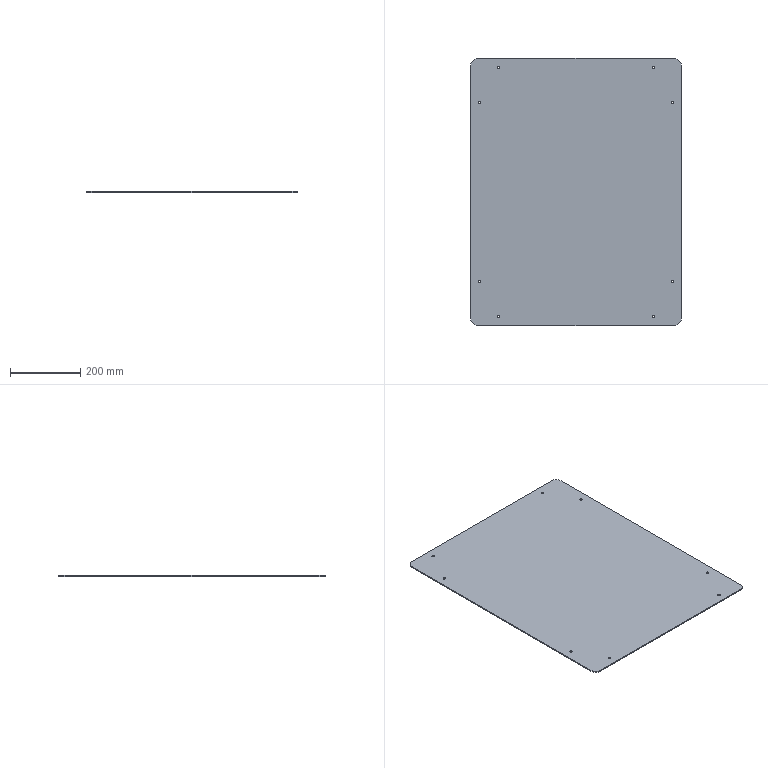Part | STEP file | 11-yakeli11 | 1 solid | 26 faces | box 600 x 760 x 3 mm | volume 1366046 mm3 | cylinder 20 | plane 6 | commonest cylinder face diameters 7 x16 40 x4
STEP:
#1=CARTESIAN_POINT('',(-216.5,-355.,0.));
#2=VERTEX_POINT('',#1);
#3=CARTESIAN_POINT('',(-223.5,-355.,0.));
#4=VERTEX_POINT('',#3);
#5=CARTESIAN_POINT('',(-220.,-355.,0.));
#6=DIRECTION('',(0.,0.,-1.));
#7=DIRECTION('',(1.,0.,0.));
#8=AXIS2_PLACEMENT_3D('',#5,#6,#7);
#9=CIRCLE('',#8,3.5);
#10=EDGE_CURVE('',#2,#4,#9,.T.);
#11=ORIENTED_EDGE('',*,*,#10,.F.);
#12=CARTESIAN_POINT('',(-216.5,-355.,-3.));
#13=VERTEX_POINT('',#12);
#14=CARTESIAN_POINT('',(-216.5,-355.,0.));
#15=DIRECTION('',(0.,0.,-1.));
#16=VECTOR('',#15,1000.);
#17=LINE('',#14,#16);
#18=EDGE_CURVE('',#2,#13,#17,.T.);
#19=ORIENTED_EDGE('',*,*,#18,.T.);
#20=CARTESIAN_POINT('',(-223.5,-355.,-3.));
#21=VERTEX_POINT('',#20);
#22=CARTESIAN_POINT('',(-220.,-355.,-3.));
#23=DIRECTION('',(0.,0.,-1.));
#24=DIRECTION('',(1.,0.,0.));
#25=AXIS2_PLACEMENT_3D('',#22,#23,#24);
#26=CIRCLE('',#25,3.5);
#27=EDGE_CURVE('',#13,#21,#26,.T.);
#28=ORIENTED_EDGE('',*,*,#27,.T.);
#29=CARTESIAN_POINT('',(-223.5,-355.,0.));
#30=DIRECTION('',(0.,0.,-1.));
#31=VECTOR('',#30,1000.);
#32=LINE('',#29,#31);
#33=EDGE_CURVE('',#4,#21,#32,.T.);
#34=ORIENTED_EDGE('',*,*,#33,.F.);
#35=EDGE_LOOP('',(#11,#19,#28,#34));
#36=FACE_OUTER_BOUND('',#35,.T.);
#37=CARTESIAN_POINT('',(-220.,-355.,0.));
#38=DIRECTION('',(0.,0.,-1.));
#39=DIRECTION('',(-1.,0.,0.));
#40=AXIS2_PLACEMENT_3D('',#37,#38,#39);
#41=CYLINDRICAL_SURFACE('',#40,3.5);
#42=ADVANCED_FACE('',(#36),#41,.F.);
#43=CARTESIAN_POINT('',(223.5,-355.,0.));
#44=VERTEX_POINT('',#43);
#45=CARTESIAN_POINT('',(216.5,-355.,0.));
#46=VERTEX_POINT('',#45);
#47=CARTESIAN_POINT('',(220.,-355.,0.));
#48=DIRECTION('',(0.,0.,-1.));
#49=DIRECTION('',(1.,0.,0.));
#50=AXIS2_PLACEMENT_3D('',#47,#48,#49);
#51=CIRCLE('',#50,3.5);
#52=EDGE_CURVE('',#44,#46,#51,.T.);
#53=ORIENTED_EDGE('',*,*,#52,.F.);
#54=CARTESIAN_POINT('',(223.5,-355.,-3.));
#55=VERTEX_POINT('',#54);
#56=CARTESIAN_POINT('',(223.5,-355.,0.));
#57=DIRECTION('',(0.,0.,-1.));
#58=VECTOR('',#57,1000.);
#59=LINE('',#56,#58);
#60=EDGE_CURVE('',#44,#55,#59,.T.);
#61=ORIENTED_EDGE('',*,*,#60,.T.);
#62=CARTESIAN_POINT('',(216.5,-355.,-3.));
#63=VERTEX_POINT('',#62);
#64=CARTESIAN_POINT('',(220.,-355.,-3.));
#65=DIRECTION('',(0.,0.,-1.));
#66=DIRECTION('',(1.,0.,0.));
#67=AXIS2_PLACEMENT_3D('',#64,#65,#66);
#68=CIRCLE('',#67,3.5);
#69=EDGE_CURVE('',#55,#63,#68,.T.);
#70=ORIENTED_EDGE('',*,*,#69,.T.);
#71=CARTESIAN_POINT('',(216.5,-355.,0.));
#72=DIRECTION('',(0.,0.,-1.));
#73=VECTOR('',#72,1000.);
#74=LINE('',#71,#73);
#75=EDGE_CURVE('',#46,#63,#74,.T.);
#76=ORIENTED_EDGE('',*,*,#75,.F.);
#77=EDGE_LOOP('',(#53,#61,#70,#76));
#78=FACE_OUTER_BOUND('',#77,.T.);
#79=CARTESIAN_POINT('',(220.,-355.,0.));
#80=DIRECTION('',(0.,0.,-1.));
#81=DIRECTION('',(-1.,0.,0.));
#82=AXIS2_PLACEMENT_3D('',#79,#80,#81);
#83=CYLINDRICAL_SURFACE('',#82,3.5);
#84=ADVANCED_FACE('',(#78),#83,.F.);
#85=CARTESIAN_POINT('',(223.5,355.,0.));
#86=VERTEX_POINT('',#85);
#87=CARTESIAN_POINT('',(216.5,355.,0.));
#88=VERTEX_POINT('',#87);
#89=CARTESIAN_POINT('',(220.,355.,0.));
#90=DIRECTION('',(0.,0.,-1.));
#91=DIRECTION('',(-1.,0.,0.));
#92=AXIS2_PLACEMENT_3D('',#89,#90,#91);
#93=CIRCLE('',#92,3.5);
#94=EDGE_CURVE('',#86,#88,#93,.T.);
#95=ORIENTED_EDGE('',*,*,#94,.F.);
#96=CARTESIAN_POINT('',(223.5,355.,-3.));
#97=VERTEX_POINT('',#96);
#98=CARTESIAN_POINT('',(223.5,355.,0.));
#99=DIRECTION('',(0.,0.,-1.));
#100=VECTOR('',#99,1000.);
#101=LINE('',#98,#100);
#102=EDGE_CURVE('',#86,#97,#101,.T.);
#103=ORIENTED_EDGE('',*,*,#102,.T.);
#104=CARTESIAN_POINT('',(216.5,355.,-3.));
#105=VERTEX_POINT('',#104);
#106=CARTESIAN_POINT('',(220.,355.,-3.));
#107=DIRECTION('',(0.,0.,-1.));
#108=DIRECTION('',(-1.,0.,0.));
#109=AXIS2_PLACEMENT_3D('',#106,#107,#108);
#110=CIRCLE('',#109,3.5);
#111=EDGE_CURVE('',#97,#105,#110,.T.);
#112=ORIENTED_EDGE('',*,*,#111,.T.);
#113=CARTESIAN_POINT('',(216.5,355.,0.));
#114=DIRECTION('',(0.,0.,-1.));
#115=VECTOR('',#114,1000.);
#116=LINE('',#113,#115);
#117=EDGE_CURVE('',#88,#105,#116,.T.);
#118=ORIENTED_EDGE('',*,*,#117,.F.);
#119=EDGE_LOOP('',(#95,#103,#112,#118));
#120=FACE_OUTER_BOUND('',#119,.T.);
#121=CARTESIAN_POINT('',(220.,355.,0.));
#122=DIRECTION('',(0.,0.,-1.));
#123=DIRECTION('',(-1.,0.,0.));
#124=AXIS2_PLACEMENT_3D('',#121,#122,#123);
#125=CYLINDRICAL_SURFACE('',#124,3.5);
#126=ADVANCED_FACE('',(#120),#125,.F.);
#127=CARTESIAN_POINT('',(-216.5,355.,0.));
#128=VERTEX_POINT('',#127);
#129=CARTESIAN_POINT('',(-223.5,355.,0.));
#130=VERTEX_POINT('',#129);
#131=CARTESIAN_POINT('',(-220.,355.,0.));
#132=DIRECTION('',(0.,0.,-1.));
#133=DIRECTION('',(-1.,0.,0.));
#134=AXIS2_PLACEMENT_3D('',#131,#132,#133);
#135=CIRCLE('',#134,3.5);
#136=EDGE_CURVE('',#128,#130,#135,.T.);
#137=ORIENTED_EDGE('',*,*,#136,.F.);
#138=CARTESIAN_POINT('',(-216.5,355.,-3.));
#139=VERTEX_POINT('',#138);
#140=CARTESIAN_POINT('',(-216.5,355.,0.));
#141=DIRECTION('',(0.,0.,-1.));
#142=VECTOR('',#141,1000.);
#143=LINE('',#140,#142);
#144=EDGE_CURVE('',#128,#139,#143,.T.);
#145=ORIENTED_EDGE('',*,*,#144,.T.);
#146=CARTESIAN_POINT('',(-223.5,355.,-3.));
#147=VERTEX_POINT('',#146);
#148=CARTESIAN_POINT('',(-220.,355.,-3.));
#149=DIRECTION('',(0.,0.,-1.));
#150=DIRECTION('',(-1.,0.,0.));
#151=AXIS2_PLACEMENT_3D('',#148,#149,#150);
#152=CIRCLE('',#151,3.5);
#153=EDGE_CURVE('',#139,#147,#152,.T.);
#154=ORIENTED_EDGE('',*,*,#153,.T.);
#155=CARTESIAN_POINT('',(-223.5,355.,0.));
#156=DIRECTION('',(0.,0.,-1.));
#157=VECTOR('',#156,1000.);
#158=LINE('',#155,#157);
#159=EDGE_CURVE('',#130,#147,#158,.T.);
#160=ORIENTED_EDGE('',*,*,#159,.F.);
#161=EDGE_LOOP('',(#137,#145,#154,#160));
#162=FACE_OUTER_BOUND('',#161,.T.);
#163=CARTESIAN_POINT('',(-220.,355.,0.));
#164=DIRECTION('',(0.,0.,-1.));
#165=DIRECTION('',(-1.,0.,0.));
#166=AXIS2_PLACEMENT_3D('',#163,#164,#165);
#167=CYLINDRICAL_SURFACE('',#166,3.5);
#168=ADVANCED_FACE('',(#162),#167,.F.);
#169=CARTESIAN_POINT('',(278.5,255.,0.));
#170=VERTEX_POINT('',#169);
#171=CARTESIAN_POINT('',(271.5,255.,0.));
#172=VERTEX_POINT('',#171);
#173=CARTESIAN_POINT('',(275.,255.,0.));
#174=DIRECTION('',(0.,0.,-1.));
#175=DIRECTION('',(-1.,0.,0.));
#176=AXIS2_PLACEMENT_3D('',#173,#174,#175);
#177=CIRCLE('',#176,3.5);
#178=EDGE_CURVE('',#170,#172,#177,.T.);
#179=ORIENTED_EDGE('',*,*,#178,.F.);
#180=CARTESIAN_POINT('',(278.5,255.,-3.));
#181=VERTEX_POINT('',#180);
#182=CARTESIAN_POINT('',(278.5,255.,0.));
#183=DIRECTION('',(0.,0.,-1.));
#184=VECTOR('',#183,1000.);
#185=LINE('',#182,#184);
#186=EDGE_CURVE('',#170,#181,#185,.T.);
#187=ORIENTED_EDGE('',*,*,#186,.T.);
#188=CARTESIAN_POINT('',(271.5,255.,-3.));
#189=VERTEX_POINT('',#188);
#190=CARTESIAN_POINT('',(275.,255.,-3.));
#191=DIRECTION('',(0.,0.,-1.));
#192=DIRECTION('',(-1.,0.,0.));
#193=AXIS2_PLACEMENT_3D('',#190,#191,#192);
#194=CIRCLE('',#193,3.5);
#195=EDGE_CURVE('',#181,#189,#194,.T.);
#196=ORIENTED_EDGE('',*,*,#195,.T.);
#197=CARTESIAN_POINT('',(271.5,255.,0.));
#198=DIRECTION('',(0.,0.,-1.));
#199=VECTOR('',#198,1000.);
#200=LINE('',#197,#199);
#201=EDGE_CURVE('',#172,#189,#200,.T.);
#202=ORIENTED_EDGE('',*,*,#201,.F.);
#203=EDGE_LOOP('',(#179,#187,#196,#202));
#204=FACE_OUTER_BOUND('',#203,.T.);
#205=CARTESIAN_POINT('',(275.,255.,0.));
#206=DIRECTION('',(0.,0.,-1.));
#207=DIRECTION('',(-1.,0.,0.));
#208=AXIS2_PLACEMENT_3D('',#205,#206,#207);
#209=CYLINDRICAL_SURFACE('',#208,3.5);
#210=ADVANCED_FACE('',(#204),#209,.F.);
#211=CARTESIAN_POINT('',(278.5,-255.,0.));
#212=VERTEX_POINT('',#211);
#213=CARTESIAN_POINT('',(271.5,-255.,0.));
#214=VERTEX_POINT('',#213);
#215=CARTESIAN_POINT('',(275.,-255.,0.));
#216=DIRECTION('',(0.,0.,-1.));
#217=DIRECTION('',(-1.,0.,0.));
#218=AXIS2_PLACEMENT_3D('',#215,#216,#217);
#219=CIRCLE('',#218,3.5);
#220=EDGE_CURVE('',#212,#214,#219,.T.);
#221=ORIENTED_EDGE('',*,*,#220,.F.);
#222=CARTESIAN_POINT('',(278.5,-255.,-3.));
#223=VERTEX_POINT('',#222);
#224=CARTESIAN_POINT('',(278.5,-255.,0.));
#225=DIRECTION('',(0.,0.,-1.));
#226=VECTOR('',#225,1000.);
#227=LINE('',#224,#226);
#228=EDGE_CURVE('',#212,#223,#227,.T.);
#229=ORIENTED_EDGE('',*,*,#228,.T.);
#230=CARTESIAN_POINT('',(271.5,-255.,-3.));
#231=VERTEX_POINT('',#230);
#232=CARTESIAN_POINT('',(275.,-255.,-3.));
#233=DIRECTION('',(0.,0.,-1.));
#234=DIRECTION('',(-1.,0.,0.));
#235=AXIS2_PLACEMENT_3D('',#232,#233,#234);
#236=CIRCLE('',#235,3.5);
#237=EDGE_CURVE('',#223,#231,#236,.T.);
#238=ORIENTED_EDGE('',*,*,#237,.T.);
#239=CARTESIAN_POINT('',(271.5,-255.,0.));
#240=DIRECTION('',(0.,0.,-1.));
#241=VECTOR('',#240,1000.);
#242=LINE('',#239,#241);
#243=EDGE_CURVE('',#214,#231,#242,.T.);
#244=ORIENTED_EDGE('',*,*,#243,.F.);
#245=EDGE_LOOP('',(#221,#229,#238,#244));
#246=FACE_OUTER_BOUND('',#245,.T.);
#247=CARTESIAN_POINT('',(275.,-255.,0.));
#248=DIRECTION('',(0.,0.,-1.));
#249=DIRECTION('',(-1.,0.,0.));
#250=AXIS2_PLACEMENT_3D('',#247,#248,#249);
#251=CYLINDRICAL_SURFACE('',#250,3.5);
#252=ADVANCED_FACE('',(#246),#251,.F.);
#253=CARTESIAN_POINT('',(-271.5,-255.,0.));
#254=VERTEX_POINT('',#253);
#255=CARTESIAN_POINT('',(-278.5,-255.,0.));
#256=VERTEX_POINT('',#255);
#257=CARTESIAN_POINT('',(-275.,-255.,0.));
#258=DIRECTION('',(0.,0.,-1.));
#259=DIRECTION('',(-1.,0.,0.));
#260=AXIS2_PLACEMENT_3D('',#257,#258,#259);
#261=CIRCLE('',#260,3.5);
#262=EDGE_CURVE('',#254,#256,#261,.T.);
#263=ORIENTED_EDGE('',*,*,#262,.F.);
#264=CARTESIAN_POINT('',(-271.5,-255.,-3.));
#265=VERTEX_POINT('',#264);
#266=CARTESIAN_POINT('',(-271.5,-255.,0.));
#267=DIRECTION('',(0.,0.,-1.));
#268=VECTOR('',#267,1000.);
#269=LINE('',#266,#268);
#270=EDGE_CURVE('',#254,#265,#269,.T.);
#271=ORIENTED_EDGE('',*,*,#270,.T.);
#272=CARTESIAN_POINT('',(-278.5,-255.,-3.));
#273=VERTEX_POINT('',#272);
#274=CARTESIAN_POINT('',(-275.,-255.,-3.));
#275=DIRECTION('',(0.,0.,-1.));
#276=DIRECTION('',(-1.,0.,0.));
#277=AXIS2_PLACEMENT_3D('',#274,#275,#276);
#278=CIRCLE('',#277,3.5);
#279=EDGE_CURVE('',#265,#273,#278,.T.);
#280=ORIENTED_EDGE('',*,*,#279,.T.);
#281=CARTESIAN_POINT('',(-278.5,-255.,0.));
#282=DIRECTION('',(0.,0.,-1.));
#283=VECTOR('',#282,1000.);
#284=LINE('',#281,#283);
#285=EDGE_CURVE('',#256,#273,#284,.T.);
#286=ORIENTED_EDGE('',*,*,#285,.F.);
#287=EDGE_LOOP('',(#263,#271,#280,#286));
#288=FACE_OUTER_BOUND('',#287,.T.);
#289=CARTESIAN_POINT('',(-275.,-255.,0.));
#290=DIRECTION('',(0.,0.,-1.));
#291=DIRECTION('',(-1.,0.,0.));
#292=AXIS2_PLACEMENT_3D('',#289,#290,#291);
#293=CYLINDRICAL_SURFACE('',#292,3.5);
#294=ADVANCED_FACE('',(#288),#293,.F.);
#295=CARTESIAN_POINT('',(-271.5,255.,0.));
#296=VERTEX_POINT('',#295);
#297=CARTESIAN_POINT('',(-278.5,255.,0.));
#298=VERTEX_POINT('',#297);
#299=CARTESIAN_POINT('',(-275.,255.,0.));
#300=DIRECTION('',(0.,0.,-1.));
#301=DIRECTION('',(-1.,0.,0.));
#302=AXIS2_PLACEMENT_3D('',#299,#300,#301);
#303=CIRCLE('',#302,3.5);
#304=EDGE_CURVE('',#296,#298,#303,.T.);
#305=ORIENTED_EDGE('',*,*,#304,.F.);
#306=CARTESIAN_POINT('',(-271.5,255.,-3.));
#307=VERTEX_POINT('',#306);
#308=CARTESIAN_POINT('',(-271.5,255.,0.));
#309=DIRECTION('',(0.,0.,-1.));
#310=VECTOR('',#309,1000.);
#311=LINE('',#308,#310);
#312=EDGE_CURVE('',#296,#307,#311,.T.);
#313=ORIENTED_EDGE('',*,*,#312,.T.);
#314=CARTESIAN_POINT('',(-278.5,255.,-3.));
#315=VERTEX_POINT('',#314);
#316=CARTESIAN_POINT('',(-275.,255.,-3.));
#317=DIRECTION('',(0.,0.,-1.));
#318=DIRECTION('',(-1.,0.,0.));
#319=AXIS2_PLACEMENT_3D('',#316,#317,#318);
#320=CIRCLE('',#319,3.5);
#321=EDGE_CURVE('',#307,#315,#320,.T.);
#322=ORIENTED_EDGE('',*,*,#321,.T.);
#323=CARTESIAN_POINT('',(-278.5,255.,0.));
#324=DIRECTION('',(0.,0.,-1.));
#325=VECTOR('',#324,1000.);
#326=LINE('',#323,#325);
#327=EDGE_CURVE('',#298,#315,#326,.T.);
#328=ORIENTED_EDGE('',*,*,#327,.F.);
#329=EDGE_LOOP('',(#305,#313,#322,#328));
#330=FACE_OUTER_BOUND('',#329,.T.);
#331=CARTESIAN_POINT('',(-275.,255.,0.));
#332=DIRECTION('',(0.,0.,-1.));
#333=DIRECTION('',(-1.,0.,0.));
#334=AXIS2_PLACEMENT_3D('',#331,#332,#333);
#335=CYLINDRICAL_SURFACE('',#334,3.5);
#336=ADVANCED_FACE('',(#330),#335,.F.);
#337=CARTESIAN_POINT('',(300.,-360.,0.));
#338=VERTEX_POINT('',#337);
#339=CARTESIAN_POINT('',(300.,360.,0.));
#340=VERTEX_POINT('',#339);
#341=CARTESIAN_POINT('',(300.,380.,0.));
#342=DIRECTION('',(0.,1.,0.));
#343=VECTOR('',#342,1000.);
#344=LINE('',#341,#343);
#345=EDGE_CURVE('',#338,#340,#344,.T.);
#346=ORIENTED_EDGE('',*,*,#345,.F.);
#347=CARTESIAN_POINT('',(300.,-360.,-3.));
#348=VERTEX_POINT('',#347);
#349=CARTESIAN_POINT('',(300.,-360.,-3.));
#350=DIRECTION('',(0.,0.,-1.));
#351=VECTOR('',#350,1000.);
#352=LINE('',#349,#351);
#353=EDGE_CURVE('',#338,#348,#352,.T.);
#354=ORIENTED_EDGE('',*,*,#353,.T.);
#355=CARTESIAN_POINT('',(300.,360.,-3.));
#356=VERTEX_POINT('',#355);
#357=CARTESIAN_POINT('',(300.,380.,-3.));
#358=DIRECTION('',(0.,1.,0.));
#359=VECTOR('',#358,1000.);
#360=LINE('',#357,#359);
#361=EDGE_CURVE('',#348,#356,#360,.T.);
#362=ORIENTED_EDGE('',*,*,#361,.T.);
#363=CARTESIAN_POINT('',(300.,360.,-3.));
#364=DIRECTION('',(0.,0.,1.));
#365=VECTOR('',#364,1000.);
#366=LINE('',#363,#365);
#367=EDGE_CURVE('',#356,#340,#366,.T.);
#368=ORIENTED_EDGE('',*,*,#367,.T.);
#369=EDGE_LOOP('',(#346,#354,#362,#368));
#370=FACE_OUTER_BOUND('',#369,.T.);
#371=CARTESIAN_POINT('',(300.,380.,-3.));
#372=DIRECTION('',(1.,0.,0.));
#373=DIRECTION('',(0.,1.,0.));
#374=AXIS2_PLACEMENT_3D('',#371,#372,#373);
#375=PLANE('',#374);
#376=ADVANCED_FACE('',(#370),#375,.T.);
#377=CARTESIAN_POINT('',(-280.,-380.,0.));
#378=VERTEX_POINT('',#377);
#379=CARTESIAN_POINT('',(280.,-380.,0.));
#380=VERTEX_POINT('',#379);
#381=CARTESIAN_POINT('',(-300.,-380.,0.));
#382=DIRECTION('',(1.,0.,0.));
#383=VECTOR('',#382,1000.);
#384=LINE('',#381,#383);
#385=EDGE_CURVE('',#378,#380,#384,.T.);
#386=ORIENTED_EDGE('',*,*,#385,.F.);
#387=CARTESIAN_POINT('',(-280.,-380.,-3.));
#388=VERTEX_POINT('',#387);
#389=CARTESIAN_POINT('',(-280.,-380.,-3.));
#390=DIRECTION('',(0.,0.,-1.));
#391=VECTOR('',#390,1000.);
#392=LINE('',#389,#391);
#393=EDGE_CURVE('',#378,#388,#392,.T.);
#394=ORIENTED_EDGE('',*,*,#393,.T.);
#395=CARTESIAN_POINT('',(280.,-380.,-3.));
#396=VERTEX_POINT('',#395);
#397=CARTESIAN_POINT('',(-300.,-380.,-3.));
#398=DIRECTION('',(1.,0.,0.));
#399=VECTOR('',#398,1000.);
#400=LINE('',#397,#399);
#401=EDGE_CURVE('',#388,#396,#400,.T.);
#402=ORIENTED_EDGE('',*,*,#401,.T.);
#403=CARTESIAN_POINT('',(280.,-380.,-3.));
#404=DIRECTION('',(0.,0.,1.));
#405=VECTOR('',#404,1000.);
#406=LINE('',#403,#405);
#407=EDGE_CURVE('',#396,#380,#406,.T.);
#408=ORIENTED_EDGE('',*,*,#407,.T.);
#409=EDGE_LOOP('',(#386,#394,#402,#408));
#410=FACE_OUTER_BOUND('',#409,.T.);
#411=CARTESIAN_POINT('',(-300.,-380.,-3.));
#412=DIRECTION('',(0.,-1.,0.));
#413=DIRECTION('',(0.,0.,-1.));
#414=AXIS2_PLACEMENT_3D('',#411,#412,#413);
#415=PLANE('',#414);
#416=ADVANCED_FACE('',(#410),#415,.T.);
#417=CARTESIAN_POINT('',(-300.,360.,-3.));
#418=VERTEX_POINT('',#417);
#419=CARTESIAN_POINT('',(-300.,-360.,-3.));
#420=VERTEX_POINT('',#419);
#421=CARTESIAN_POINT('',(-300.,380.,-3.));
#422=DIRECTION('',(0.,-1.,0.));
#423=VECTOR('',#422,1000.);
#424=LINE('',#421,#423);
#425=EDGE_CURVE('',#418,#420,#424,.T.);
#426=ORIENTED_EDGE('',*,*,#425,.T.);
#427=CARTESIAN_POINT('',(-300.,-360.,0.));
#428=VERTEX_POINT('',#427);
#429=CARTESIAN_POINT('',(-300.,-360.,-3.));
#430=DIRECTION('',(0.,0.,1.));
#431=VECTOR('',#430,1000.);
#432=LINE('',#429,#431);
#433=EDGE_CURVE('',#420,#428,#432,.T.);
#434=ORIENTED_EDGE('',*,*,#433,.T.);
#435=CARTESIAN_POINT('',(-300.,360.,0.));
#436=VERTEX_POINT('',#435);
#437=CARTESIAN_POINT('',(-300.,380.,0.));
#438=DIRECTION('',(0.,-1.,0.));
#439=VECTOR('',#438,1000.);
#440=LINE('',#437,#439);
#441=EDGE_CURVE('',#436,#428,#440,.T.);
#442=ORIENTED_EDGE('',*,*,#441,.F.);
#443=CARTESIAN_POINT('',(-300.,360.,-3.));
#444=DIRECTION('',(0.,0.,-1.));
#445=VECTOR('',#444,1000.);
#446=LINE('',#443,#445);
#447=EDGE_CURVE('',#436,#418,#446,.T.);
#448=ORIENTED_EDGE('',*,*,#447,.T.);
#449=EDGE_LOOP('',(#426,#434,#442,#448));
#450=FACE_OUTER_BOUND('',#449,.T.);
#451=CARTESIAN_POINT('',(-300.,380.,-3.));
#452=DIRECTION('',(-1.,0.,0.));
#453=DIRECTION('',(0.,-1.,0.));
#454=AXIS2_PLACEMENT_3D('',#451,#452,#453);
#455=PLANE('',#454);
#456=ADVANCED_FACE('',(#450),#455,.T.);
#457=CARTESIAN_POINT('',(280.,380.,0.));
#458=VERTEX_POINT('',#457);
#459=CARTESIAN_POINT('',(-280.,380.,0.));
#460=VERTEX_POINT('',#459);
#461=CARTESIAN_POINT('',(-300.,380.,0.));
#462=DIRECTION('',(-1.,0.,0.));
#463=VECTOR('',#462,1000.);
#464=LINE('',#461,#463);
#465=EDGE_CURVE('',#458,#460,#464,.T.);
#466=ORIENTED_EDGE('',*,*,#465,.F.);
#467=CARTESIAN_POINT('',(280.,380.,-3.));
#468=VERTEX_POINT('',#467);
#469=CARTESIAN_POINT('',(280.,380.,-3.));
#470=DIRECTION('',(0.,0.,-1.));
#471=VECTOR('',#470,1000.);
#472=LINE('',#469,#471);
#473=EDGE_CURVE('',#458,#468,#472,.T.);
#474=ORIENTED_EDGE('',*,*,#473,.T.);
#475=CARTESIAN_POINT('',(-280.,380.,-3.));
#476=VERTEX_POINT('',#475);
#477=CARTESIAN_POINT('',(-300.,380.,-3.));
#478=DIRECTION('',(-1.,0.,0.));
#479=VECTOR('',#478,1000.);
#480=LINE('',#477,#479);
#481=EDGE_CURVE('',#468,#476,#480,.T.);
#482=ORIENTED_EDGE('',*,*,#481,.T.);
#483=CARTESIAN_POINT('',(-280.,380.,-3.));
#484=DIRECTION('',(0.,0.,1.));
#485=VECTOR('',#484,1000.);
#486=LINE('',#483,#485);
#487=EDGE_CURVE('',#476,#460,#486,.T.);
#488=ORIENTED_EDGE('',*,*,#487,.T.);
#489=EDGE_LOOP('',(#466,#474,#482,#488));
#490=FACE_OUTER_BOUND('',#489,.T.);
#491=CARTESIAN_POINT('',(-300.,380.,-3.));
#492=DIRECTION('',(0.,1.,0.));
#493=DIRECTION('',(0.,0.,1.));
#494=AXIS2_PLACEMENT_3D('',#491,#492,#493);
#495=PLANE('',#494);
#496=ADVANCED_FACE('',(#490),#495,.T.);
#497=CARTESIAN_POINT('',(-220.,-355.,-3.));
#498=DIRECTION('',(0.,0.,-1.));
#499=DIRECTION('',(1.,0.,0.));
#500=AXIS2_PLACEMENT_3D('',#497,#498,#499);
#501=CIRCLE('',#500,3.5);
#502=EDGE_CURVE('',#21,#13,#501,.T.);
#503=ORIENTED_EDGE('',*,*,#502,.F.);
#504=ORIENTED_EDGE('',*,*,#27,.F.);
#505=EDGE_LOOP('',(#503,#504));
#506=FACE_BOUND('',#505,.T.);
#507=CARTESIAN_POINT('',(220.,-355.,-3.));
#508=DIRECTION('',(0.,0.,-1.));
#509=DIRECTION('',(1.,0.,0.));
#510=AXIS2_PLACEMENT_3D('',#507,#508,#509);
#511=CIRCLE('',#510,3.5);
#512=EDGE_CURVE('',#63,#55,#511,.T.);
#513=ORIENTED_EDGE('',*,*,#512,.F.);
#514=ORIENTED_EDGE('',*,*,#69,.F.);
#515=EDGE_LOOP('',(#513,#514));
#516=FACE_BOUND('',#515,.T.);
#517=CARTESIAN_POINT('',(220.,355.,-3.));
#518=DIRECTION('',(0.,0.,-1.));
#519=DIRECTION('',(-1.,0.,0.));
#520=AXIS2_PLACEMENT_3D('',#517,#518,#519);
#521=CIRCLE('',#520,3.5);
#522=EDGE_CURVE('',#105,#97,#521,.T.);
#523=ORIENTED_EDGE('',*,*,#522,.F.);
#524=ORIENTED_EDGE('',*,*,#111,.F.);
#525=EDGE_LOOP('',(#523,#524));
#526=FACE_BOUND('',#525,.T.);
#527=CARTESIAN_POINT('',(-220.,355.,-3.));
#528=DIRECTION('',(0.,0.,-1.));
#529=DIRECTION('',(-1.,0.,0.));
#530=AXIS2_PLACEMENT_3D('',#527,#528,#529);
#531=CIRCLE('',#530,3.5);
#532=EDGE_CURVE('',#147,#139,#531,.T.);
#533=ORIENTED_EDGE('',*,*,#532,.F.);
#534=ORIENTED_EDGE('',*,*,#153,.F.);
#535=EDGE_LOOP('',(#533,#534));
#536=FACE_BOUND('',#535,.T.);
#537=CARTESIAN_POINT('',(275.,255.,-3.));
#538=DIRECTION('',(0.,0.,-1.));
#539=DIRECTION('',(-1.,0.,0.));
#540=AXIS2_PLACEMENT_3D('',#537,#538,#539);
#541=CIRCLE('',#540,3.5);
#542=EDGE_CURVE('',#189,#181,#541,.T.);
#543=ORIENTED_EDGE('',*,*,#542,.F.);
#544=ORIENTED_EDGE('',*,*,#195,.F.);
#545=EDGE_LOOP('',(#543,#544));
#546=FACE_BOUND('',#545,.T.);
#547=CARTESIAN_POINT('',(275.,-255.,-3.));
#548=DIRECTION('',(0.,0.,-1.));
#549=DIRECTION('',(-1.,0.,0.));
#550=AXIS2_PLACEMENT_3D('',#547,#548,#549);
#551=CIRCLE('',#550,3.5);
#552=EDGE_CURVE('',#231,#223,#551,.T.);
#553=ORIENTED_EDGE('',*,*,#552,.F.);
#554=ORIENTED_EDGE('',*,*,#237,.F.);
#555=EDGE_LOOP('',(#553,#554));
#556=FACE_BOUND('',#555,.T.);
#557=CARTESIAN_POINT('',(-275.,-255.,-3.));
#558=DIRECTION('',(0.,0.,-1.));
#559=DIRECTION('',(-1.,0.,0.));
#560=AXIS2_PLACEMENT_3D('',#557,#558,#559);
#561=CIRCLE('',#560,3.5);
#562=EDGE_CURVE('',#273,#265,#561,.T.);
#563=ORIENTED_EDGE('',*,*,#562,.F.);
#564=ORIENTED_EDGE('',*,*,#279,.F.);
#565=EDGE_LOOP('',(#563,#564));
#566=FACE_BOUND('',#565,.T.);
#567=CARTESIAN_POINT('',(-275.,255.,-3.));
#568=DIRECTION('',(0.,0.,-1.));
#569=DIRECTION('',(-1.,0.,0.));
#570=AXIS2_PLACEMENT_3D('',#567,#568,#569);
#571=CIRCLE('',#570,3.5);
#572=EDGE_CURVE('',#315,#307,#571,.T.);
#573=ORIENTED_EDGE('',*,*,#572,.F.);
#574=ORIENTED_EDGE('',*,*,#321,.F.);
#575=EDGE_LOOP('',(#573,#574));
#576=FACE_BOUND('',#575,.T.);
#577=ORIENTED_EDGE('',*,*,#401,.F.);
#578=CARTESIAN_POINT('',(-280.,-360.,-3.));
#579=DIRECTION('',(0.,0.,-1.));
#580=DIRECTION('',(1.,0.,0.));
#581=AXIS2_PLACEMENT_3D('',#578,#579,#580);
#582=CIRCLE('',#581,20.);
#583=EDGE_CURVE('',#388,#420,#582,.T.);
#584=ORIENTED_EDGE('',*,*,#583,.T.);
#585=ORIENTED_EDGE('',*,*,#425,.F.);
#586=CARTESIAN_POINT('',(-280.,360.,-3.));
#587=DIRECTION('',(0.,0.,-1.));
#588=DIRECTION('',(1.,0.,0.));
#589=AXIS2_PLACEMENT_3D('',#586,#587,#588);
#590=CIRCLE('',#589,20.);
#591=EDGE_CURVE('',#418,#476,#590,.T.);
#592=ORIENTED_EDGE('',*,*,#591,.T.);
#593=ORIENTED_EDGE('',*,*,#481,.F.);
#594=CARTESIAN_POINT('',(280.,360.,-3.));
#595=DIRECTION('',(0.,0.,-1.));
#596=DIRECTION('',(1.,0.,0.));
#597=AXIS2_PLACEMENT_3D('',#594,#595,#596);
#598=CIRCLE('',#597,20.);
#599=EDGE_CURVE('',#468,#356,#598,.T.);
#600=ORIENTED_EDGE('',*,*,#599,.T.);
#601=ORIENTED_EDGE('',*,*,#361,.F.);
#602=CARTESIAN_POINT('',(280.,-360.,-3.));
#603=DIRECTION('',(0.,0.,-1.));
#604=DIRECTION('',(1.,0.,0.));
#605=AXIS2_PLACEMENT_3D('',#602,#603,#604);
#606=CIRCLE('',#605,20.);
#607=EDGE_CURVE('',#348,#396,#606,.T.);
#608=ORIENTED_EDGE('',*,*,#607,.T.);
#609=EDGE_LOOP('',(#577,#584,#585,#592,#593,#600,#601,#608));
#610=FACE_OUTER_BOUND('',#609,.T.);
#611=CARTESIAN_POINT('',(0.,0.,-3.));
#612=DIRECTION('',(0.,0.,1.));
#613=DIRECTION('',(1.,0.,0.));
#614=AXIS2_PLACEMENT_3D('',#611,#612,#613);
#615=PLANE('',#614);
#616=ADVANCED_FACE('',(#506,#516,#526,#536,#546,#556,#566,#576,#610),#615,.F.);
#617=CARTESIAN_POINT('',(-220.,-355.,0.));
#618=DIRECTION('',(0.,0.,-1.));
#619=DIRECTION('',(1.,0.,0.));
#620=AXIS2_PLACEMENT_3D('',#617,#618,#619);
#621=CIRCLE('',#620,3.5);
#622=EDGE_CURVE('',#4,#2,#621,.T.);
#623=ORIENTED_EDGE('',*,*,#622,.T.);
#624=ORIENTED_EDGE('',*,*,#10,.T.);
#625=EDGE_LOOP('',(#623,#624));
#626=FACE_BOUND('',#625,.T.);
#627=CARTESIAN_POINT('',(220.,-355.,0.));
#628=DIRECTION('',(0.,0.,-1.));
#629=DIRECTION('',(1.,0.,0.));
#630=AXIS2_PLACEMENT_3D('',#627,#628,#629);
#631=CIRCLE('',#630,3.5);
#632=EDGE_CURVE('',#46,#44,#631,.T.);
#633=ORIENTED_EDGE('',*,*,#632,.T.);
#634=ORIENTED_EDGE('',*,*,#52,.T.);
#635=EDGE_LOOP('',(#633,#634));
#636=FACE_BOUND('',#635,.T.);
#637=CARTESIAN_POINT('',(220.,355.,0.));
#638=DIRECTION('',(0.,0.,-1.));
#639=DIRECTION('',(-1.,0.,0.));
#640=AXIS2_PLACEMENT_3D('',#637,#638,#639);
#641=CIRCLE('',#640,3.5);
#642=EDGE_CURVE('',#88,#86,#641,.T.);
#643=ORIENTED_EDGE('',*,*,#642,.T.);
#644=ORIENTED_EDGE('',*,*,#94,.T.);
#645=EDGE_LOOP('',(#643,#644));
#646=FACE_BOUND('',#645,.T.);
#647=CARTESIAN_POINT('',(-220.,355.,0.));
#648=DIRECTION('',(0.,0.,-1.));
#649=DIRECTION('',(-1.,0.,0.));
#650=AXIS2_PLACEMENT_3D('',#647,#648,#649);
#651=CIRCLE('',#650,3.5);
#652=EDGE_CURVE('',#130,#128,#651,.T.);
#653=ORIENTED_EDGE('',*,*,#652,.T.);
#654=ORIENTED_EDGE('',*,*,#136,.T.);
#655=EDGE_LOOP('',(#653,#654));
#656=FACE_BOUND('',#655,.T.);
#657=CARTESIAN_POINT('',(275.,255.,0.));
#658=DIRECTION('',(0.,0.,-1.));
#659=DIRECTION('',(-1.,0.,0.));
#660=AXIS2_PLACEMENT_3D('',#657,#658,#659);
#661=CIRCLE('',#660,3.5);
#662=EDGE_CURVE('',#172,#170,#661,.T.);
#663=ORIENTED_EDGE('',*,*,#662,.T.);
#664=ORIENTED_EDGE('',*,*,#178,.T.);
#665=EDGE_LOOP('',(#663,#664));
#666=FACE_BOUND('',#665,.T.);
#667=CARTESIAN_POINT('',(275.,-255.,0.));
#668=DIRECTION('',(0.,0.,-1.));
#669=DIRECTION('',(-1.,0.,0.));
#670=AXIS2_PLACEMENT_3D('',#667,#668,#669);
#671=CIRCLE('',#670,3.5);
#672=EDGE_CURVE('',#214,#212,#671,.T.);
#673=ORIENTED_EDGE('',*,*,#672,.T.);
#674=ORIENTED_EDGE('',*,*,#220,.T.);
#675=EDGE_LOOP('',(#673,#674));
#676=FACE_BOUND('',#675,.T.);
#677=CARTESIAN_POINT('',(-275.,-255.,0.));
#678=DIRECTION('',(0.,0.,-1.));
#679=DIRECTION('',(-1.,0.,0.));
#680=AXIS2_PLACEMENT_3D('',#677,#678,#679);
#681=CIRCLE('',#680,3.5);
#682=EDGE_CURVE('',#256,#254,#681,.T.);
#683=ORIENTED_EDGE('',*,*,#682,.T.);
#684=ORIENTED_EDGE('',*,*,#262,.T.);
#685=EDGE_LOOP('',(#683,#684));
#686=FACE_BOUND('',#685,.T.);
#687=CARTESIAN_POINT('',(-275.,255.,0.));
#688=DIRECTION('',(0.,0.,-1.));
#689=DIRECTION('',(-1.,0.,0.));
#690=AXIS2_PLACEMENT_3D('',#687,#688,#689);
#691=CIRCLE('',#690,3.5);
#692=EDGE_CURVE('',#298,#296,#691,.T.);
#693=ORIENTED_EDGE('',*,*,#692,.T.);
#694=ORIENTED_EDGE('',*,*,#304,.T.);
#695=EDGE_LOOP('',(#693,#694));
#696=FACE_BOUND('',#695,.T.);
#697=ORIENTED_EDGE('',*,*,#441,.T.);
#698=CARTESIAN_POINT('',(-280.,-360.,0.));
#699=DIRECTION('',(0.,0.,1.));
#700=DIRECTION('',(1.,0.,0.));
#701=AXIS2_PLACEMENT_3D('',#698,#699,#700);
#702=CIRCLE('',#701,20.);
#703=EDGE_CURVE('',#428,#378,#702,.T.);
#704=ORIENTED_EDGE('',*,*,#703,.T.);
#705=ORIENTED_EDGE('',*,*,#385,.T.);
#706=CARTESIAN_POINT('',(280.,-360.,0.));
#707=DIRECTION('',(0.,0.,1.));
#708=DIRECTION('',(1.,0.,0.));
#709=AXIS2_PLACEMENT_3D('',#706,#707,#708);
#710=CIRCLE('',#709,20.);
#711=EDGE_CURVE('',#380,#338,#710,.T.);
#712=ORIENTED_EDGE('',*,*,#711,.T.);
#713=ORIENTED_EDGE('',*,*,#345,.T.);
#714=CARTESIAN_POINT('',(280.,360.,0.));
#715=DIRECTION('',(0.,0.,1.));
#716=DIRECTION('',(1.,0.,0.));
#717=AXIS2_PLACEMENT_3D('',#714,#715,#716);
#718=CIRCLE('',#717,20.);
#719=EDGE_CURVE('',#340,#458,#718,.T.);
#720=ORIENTED_EDGE('',*,*,#719,.T.);
#721=ORIENTED_EDGE('',*,*,#465,.T.);
#722=CARTESIAN_POINT('',(-280.,360.,0.));
#723=DIRECTION('',(0.,0.,1.));
#724=DIRECTION('',(1.,0.,0.));
#725=AXIS2_PLACEMENT_3D('',#722,#723,#724);
#726=CIRCLE('',#725,20.);
#727=EDGE_CURVE('',#460,#436,#726,.T.);
#728=ORIENTED_EDGE('',*,*,#727,.T.);
#729=EDGE_LOOP('',(#697,#704,#705,#712,#713,#720,#721,#728));
#730=FACE_OUTER_BOUND('',#729,.T.);
#731=CARTESIAN_POINT('',(0.,0.,0.));
#732=DIRECTION('',(0.,0.,1.));
#733=DIRECTION('',(1.,0.,0.));
#734=AXIS2_PLACEMENT_3D('',#731,#732,#733);
#735=PLANE('',#734);
#736=ADVANCED_FACE('',(#626,#636,#646,#656,#666,#676,#686,#696,#730),#735,.T.);
#737=ORIENTED_EDGE('',*,*,#583,.F.);
#738=ORIENTED_EDGE('',*,*,#393,.F.);
#739=ORIENTED_EDGE('',*,*,#703,.F.);
#740=ORIENTED_EDGE('',*,*,#433,.F.);
#741=EDGE_LOOP('',(#737,#738,#739,#740));
#742=FACE_OUTER_BOUND('',#741,.T.);
#743=CARTESIAN_POINT('',(-280.,-360.,-3.));
#744=DIRECTION('',(0.,0.,1.));
#745=DIRECTION('',(1.,0.,0.));
#746=AXIS2_PLACEMENT_3D('',#743,#744,#745);
#747=CYLINDRICAL_SURFACE('',#746,20.);
#748=ADVANCED_FACE('',(#742),#747,.T.);
#749=ORIENTED_EDGE('',*,*,#607,.F.);
#750=ORIENTED_EDGE('',*,*,#353,.F.);
#751=ORIENTED_EDGE('',*,*,#711,.F.);
#752=ORIENTED_EDGE('',*,*,#407,.F.);
#753=EDGE_LOOP('',(#749,#750,#751,#752));
#754=FACE_OUTER_BOUND('',#753,.T.);
#755=CARTESIAN_POINT('',(280.,-360.,-3.));
#756=DIRECTION('',(0.,0.,1.));
#757=DIRECTION('',(1.,0.,0.));
#758=AXIS2_PLACEMENT_3D('',#755,#756,#757);
#759=CYLINDRICAL_SURFACE('',#758,20.);
#760=ADVANCED_FACE('',(#754),#759,.T.);
#761=ORIENTED_EDGE('',*,*,#599,.F.);
#762=ORIENTED_EDGE('',*,*,#473,.F.);
#763=ORIENTED_EDGE('',*,*,#719,.F.);
#764=ORIENTED_EDGE('',*,*,#367,.F.);
#765=EDGE_LOOP('',(#761,#762,#763,#764));
#766=FACE_OUTER_BOUND('',#765,.T.);
#767=CARTESIAN_POINT('',(280.,360.,-3.));
#768=DIRECTION('',(0.,0.,1.));
#769=DIRECTION('',(1.,0.,0.));
#770=AXIS2_PLACEMENT_3D('',#767,#768,#769);
#771=CYLINDRICAL_SURFACE('',#770,20.);
#772=ADVANCED_FACE('',(#766),#771,.T.);
#773=ORIENTED_EDGE('',*,*,#591,.F.);
#774=ORIENTED_EDGE('',*,*,#447,.F.);
#775=ORIENTED_EDGE('',*,*,#727,.F.);
#776=ORIENTED_EDGE('',*,*,#487,.F.);
#777=EDGE_LOOP('',(#773,#774,#775,#776));
#778=FACE_OUTER_BOUND('',#777,.T.);
#779=CARTESIAN_POINT('',(-280.,360.,-3.));
#780=DIRECTION('',(0.,0.,1.));
#781=DIRECTION('',(1.,0.,0.));
#782=AXIS2_PLACEMENT_3D('',#779,#780,#781);
#783=CYLINDRICAL_SURFACE('',#782,20.);
#784=ADVANCED_FACE('',(#778),#783,.T.);
#785=ORIENTED_EDGE('',*,*,#312,.F.);
#786=ORIENTED_EDGE('',*,*,#692,.F.);
#787=ORIENTED_EDGE('',*,*,#327,.T.);
#788=ORIENTED_EDGE('',*,*,#572,.T.);
#789=EDGE_LOOP('',(#785,#786,#787,#788));
#790=FACE_OUTER_BOUND('',#789,.T.);
#791=CARTESIAN_POINT('',(-275.,255.,0.));
#792=DIRECTION('',(0.,0.,-1.));
#793=DIRECTION('',(-1.,0.,0.));
#794=AXIS2_PLACEMENT_3D('',#791,#792,#793);
#795=CYLINDRICAL_SURFACE('',#794,3.5);
#796=ADVANCED_FACE('',(#790),#795,.F.);
#797=ORIENTED_EDGE('',*,*,#270,.F.);
#798=ORIENTED_EDGE('',*,*,#682,.F.);
#799=ORIENTED_EDGE('',*,*,#285,.T.);
#800=ORIENTED_EDGE('',*,*,#562,.T.);
#801=EDGE_LOOP('',(#797,#798,#799,#800));
#802=FACE_OUTER_BOUND('',#801,.T.);
#803=CARTESIAN_POINT('',(-275.,-255.,0.));
#804=DIRECTION('',(0.,0.,-1.));
#805=DIRECTION('',(-1.,0.,0.));
#806=AXIS2_PLACEMENT_3D('',#803,#804,#805);
#807=CYLINDRICAL_SURFACE('',#806,3.5);
#808=ADVANCED_FACE('',(#802),#807,.F.);
#809=ORIENTED_EDGE('',*,*,#228,.F.);
#810=ORIENTED_EDGE('',*,*,#672,.F.);
#811=ORIENTED_EDGE('',*,*,#243,.T.);
#812=ORIENTED_EDGE('',*,*,#552,.T.);
#813=EDGE_LOOP('',(#809,#810,#811,#812));
#814=FACE_OUTER_BOUND('',#813,.T.);
#815=CARTESIAN_POINT('',(275.,-255.,0.));
#816=DIRECTION('',(0.,0.,-1.));
#817=DIRECTION('',(-1.,0.,0.));
#818=AXIS2_PLACEMENT_3D('',#815,#816,#817);
#819=CYLINDRICAL_SURFACE('',#818,3.5);
#820=ADVANCED_FACE('',(#814),#819,.F.);
#821=ORIENTED_EDGE('',*,*,#186,.F.);
#822=ORIENTED_EDGE('',*,*,#662,.F.);
#823=ORIENTED_EDGE('',*,*,#201,.T.);
#824=ORIENTED_EDGE('',*,*,#542,.T.);
#825=EDGE_LOOP('',(#821,#822,#823,#824));
#826=FACE_OUTER_BOUND('',#825,.T.);
#827=CARTESIAN_POINT('',(275.,255.,0.));
#828=DIRECTION('',(0.,0.,-1.));
#829=DIRECTION('',(-1.,0.,0.));
#830=AXIS2_PLACEMENT_3D('',#827,#828,#829);
#831=CYLINDRICAL_SURFACE('',#830,3.5);
#832=ADVANCED_FACE('',(#826),#831,.F.);
#833=ORIENTED_EDGE('',*,*,#144,.F.);
#834=ORIENTED_EDGE('',*,*,#652,.F.);
#835=ORIENTED_EDGE('',*,*,#159,.T.);
#836=ORIENTED_EDGE('',*,*,#532,.T.);
#837=EDGE_LOOP('',(#833,#834,#835,#836));
#838=FACE_OUTER_BOUND('',#837,.T.);
#839=CARTESIAN_POINT('',(-220.,355.,0.));
#840=DIRECTION('',(0.,0.,-1.));
#841=DIRECTION('',(-1.,0.,0.));
#842=AXIS2_PLACEMENT_3D('',#839,#840,#841);
#843=CYLINDRICAL_SURFACE('',#842,3.5);
#844=ADVANCED_FACE('',(#838),#843,.F.);
#845=ORIENTED_EDGE('',*,*,#102,.F.);
#846=ORIENTED_EDGE('',*,*,#642,.F.);
#847=ORIENTED_EDGE('',*,*,#117,.T.);
#848=ORIENTED_EDGE('',*,*,#522,.T.);
#849=EDGE_LOOP('',(#845,#846,#847,#848));
#850=FACE_OUTER_BOUND('',#849,.T.);
#851=CARTESIAN_POINT('',(220.,355.,0.));
#852=DIRECTION('',(0.,0.,-1.));
#853=DIRECTION('',(-1.,0.,0.));
#854=AXIS2_PLACEMENT_3D('',#851,#852,#853);
#855=CYLINDRICAL_SURFACE('',#854,3.5);
#856=ADVANCED_FACE('',(#850),#855,.F.);
#857=ORIENTED_EDGE('',*,*,#60,.F.);
#858=ORIENTED_EDGE('',*,*,#632,.F.);
#859=ORIENTED_EDGE('',*,*,#75,.T.);
#860=ORIENTED_EDGE('',*,*,#512,.T.);
#861=EDGE_LOOP('',(#857,#858,#859,#860));
#862=FACE_OUTER_BOUND('',#861,.T.);
#863=CARTESIAN_POINT('',(220.,-355.,0.));
#864=DIRECTION('',(0.,0.,-1.));
#865=DIRECTION('',(-1.,0.,0.));
#866=AXIS2_PLACEMENT_3D('',#863,#864,#865);
#867=CYLINDRICAL_SURFACE('',#866,3.5);
#868=ADVANCED_FACE('',(#862),#867,.F.);
#869=ORIENTED_EDGE('',*,*,#18,.F.);
#870=ORIENTED_EDGE('',*,*,#622,.F.);
#871=ORIENTED_EDGE('',*,*,#33,.T.);
#872=ORIENTED_EDGE('',*,*,#502,.T.);
#873=EDGE_LOOP('',(#869,#870,#871,#872));
#874=FACE_OUTER_BOUND('',#873,.T.);
#875=CARTESIAN_POINT('',(-220.,-355.,0.));
#876=DIRECTION('',(0.,0.,-1.));
#877=DIRECTION('',(-1.,0.,0.));
#878=AXIS2_PLACEMENT_3D('',#875,#876,#877);
#879=CYLINDRICAL_SURFACE('',#878,3.5);
#880=ADVANCED_FACE('',(#874),#879,.F.);
#881=CLOSED_SHELL('',(#42,#84,#126,#168,#210,#252,#294,#336,#376,#416,#456,#496,#616,#736,#748,#760,#772,#784,#796,#808,#820,#832,#844,#856,#868,#880));
#882=MANIFOLD_SOLID_BREP('',#881);
#883=CARTESIAN_POINT('',(0.,0.,0.));
#884=DIRECTION('',(0.,0.,1.));
#885=DIRECTION('',(1.,0.,0.));
#886=AXIS2_PLACEMENT_3D('',#883,#884,#885);
#887=(LENGTH_UNIT()NAMED_UNIT(*)SI_UNIT(.MILLI.,.METRE.));
#888=UNCERTAINTY_MEASURE_WITH_UNIT(LENGTH_MEASURE(0.00001),#887,'','');
#889=(NAMED_UNIT(*)PLANE_ANGLE_UNIT()SI_UNIT($,.RADIAN.));
#890=(NAMED_UNIT(*)SI_UNIT($,.STERADIAN.)SOLID_ANGLE_UNIT());
#891=(GEOMETRIC_REPRESENTATION_CONTEXT(3)GLOBAL_UNCERTAINTY_ASSIGNED_CONTEXT((#888))GLOBAL_UNIT_ASSIGNED_CONTEXT((#887,#889,#890))REPRESENTATION_CONTEXT('',''));
#892=ADVANCED_BREP_SHAPE_REPRESENTATION('',(#882,#886),#891);